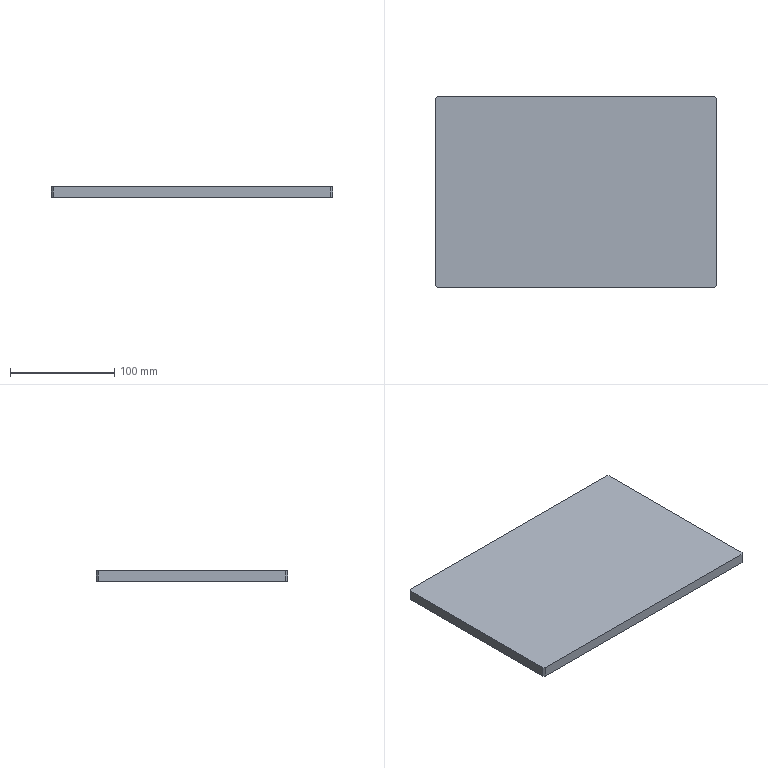Part | STEP file | 001-011-Blanking flip base plate | 1 solid | 10 faces | box 270 x 184 x 10 mm | volume 496720 mm3 | plane 10
STEP:
#1=CARTESIAN_POINT('',(0.,0.,0.));
#2=DIRECTION('',(0.,0.,1.));
#3=DIRECTION('',(1.,0.,0.));
#4=AXIS2_PLACEMENT_3D('',#1,#2,#3);
#5=CARTESIAN_POINT('',(135.,-90.,10.));
#6=VERTEX_POINT('',#5);
#7=CARTESIAN_POINT('',(135.,90.,10.));
#8=VERTEX_POINT('',#7);
#9=CARTESIAN_POINT('',(135.,-92.,10.));
#10=DIRECTION('',(0.,1.,0.));
#11=VECTOR('',#10,1.);
#12=LINE('',#9,#11);
#13=CARTESIAN_POINT('',(135.,-92.,10.));
#14=DIRECTION('',(-1.,0.,0.));
#15=DIRECTION('',(0.,-1.,0.));
#16=AXIS2_PLACEMENT_3D('',#13,#14,#15);
#17=PLANE('',#16);
#18=CARTESIAN_POINT('',(0.,0.));
#19=DIRECTION('',(-1.,0.));
#20=VECTOR('',#19,1.);
#21=LINE('',#18,#20);
#22=(GEOMETRIC_REPRESENTATION_CONTEXT(2)PARAMETRIC_REPRESENTATION_CONTEXT()REPRESENTATION_CONTEXT('',''));
#23=DEFINITIONAL_REPRESENTATION('',(#21),#22);
#24=PCURVE('',#17,#23);
#25=CARTESIAN_POINT('',(0.,0.,10.));
#26=DIRECTION('',(0.,0.,-1.));
#27=DIRECTION('',(-1.,0.,0.));
#28=AXIS2_PLACEMENT_3D('',#25,#26,#27);
#29=PLANE('',#28);
#30=CARTESIAN_POINT('',(-135.,-92.));
#31=DIRECTION('',(0.,1.));
#32=VECTOR('',#31,1.);
#33=LINE('',#30,#32);
#34=(GEOMETRIC_REPRESENTATION_CONTEXT(2)PARAMETRIC_REPRESENTATION_CONTEXT()REPRESENTATION_CONTEXT('',''));
#35=DEFINITIONAL_REPRESENTATION('',(#33),#34);
#36=PCURVE('',#29,#35);
#37=SURFACE_CURVE('',#12,(#24,#36),.PCURVE_S1.);
#38=EDGE_CURVE('',#6,#8,#37,.T.);
#39=ORIENTED_EDGE('',*,*,#38,.F.);
#40=CARTESIAN_POINT('',(135.,-90.,0.));
#41=VERTEX_POINT('',#40);
#42=CARTESIAN_POINT('',(135.,-90.,10.));
#43=DIRECTION('',(0.,0.,-1.));
#44=VECTOR('',#43,1.);
#45=LINE('',#42,#44);
#46=CARTESIAN_POINT('',(-2.,0.));
#47=DIRECTION('',(0.,-1.));
#48=VECTOR('',#47,1.);
#49=LINE('',#46,#48);
#50=(GEOMETRIC_REPRESENTATION_CONTEXT(2)PARAMETRIC_REPRESENTATION_CONTEXT()REPRESENTATION_CONTEXT('',''));
#51=DEFINITIONAL_REPRESENTATION('',(#49),#50);
#52=PCURVE('',#17,#51);
#53=CARTESIAN_POINT('',(135.,-90.,10.));
#54=DIRECTION('',(-0.7071,0.7071,0.));
#55=DIRECTION('',(0.,0.,-1.));
#56=AXIS2_PLACEMENT_3D('',#53,#54,#55);
#57=PLANE('',#56);
#58=CARTESIAN_POINT('',(0.,0.));
#59=DIRECTION('',(1.,0.));
#60=VECTOR('',#59,1.);
#61=LINE('',#58,#60);
#62=(GEOMETRIC_REPRESENTATION_CONTEXT(2)PARAMETRIC_REPRESENTATION_CONTEXT()REPRESENTATION_CONTEXT('',''));
#63=DEFINITIONAL_REPRESENTATION('',(#61),#62);
#64=PCURVE('',#57,#63);
#65=SURFACE_CURVE('',#45,(#52,#64),.PCURVE_S1.);
#66=EDGE_CURVE('',#6,#41,#65,.T.);
#67=ORIENTED_EDGE('',*,*,#66,.T.);
#68=CARTESIAN_POINT('',(135.,90.,0.));
#69=VERTEX_POINT('',#68);
#70=CARTESIAN_POINT('',(135.,-92.,0.));
#71=DIRECTION('',(0.,1.,0.));
#72=VECTOR('',#71,1.);
#73=LINE('',#70,#72);
#74=CARTESIAN_POINT('',(0.,-10.));
#75=DIRECTION('',(-1.,0.));
#76=VECTOR('',#75,1.);
#77=LINE('',#74,#76);
#78=(GEOMETRIC_REPRESENTATION_CONTEXT(2)PARAMETRIC_REPRESENTATION_CONTEXT()REPRESENTATION_CONTEXT('',''));
#79=DEFINITIONAL_REPRESENTATION('',(#77),#78);
#80=PCURVE('',#17,#79);
#81=CARTESIAN_POINT('',(0.,0.,0.));
#82=DIRECTION('',(0.,0.,-1.));
#83=DIRECTION('',(-1.,0.,0.));
#84=AXIS2_PLACEMENT_3D('',#81,#82,#83);
#85=PLANE('',#84);
#86=CARTESIAN_POINT('',(-135.,-92.));
#87=DIRECTION('',(0.,1.));
#88=VECTOR('',#87,1.);
#89=LINE('',#86,#88);
#90=(GEOMETRIC_REPRESENTATION_CONTEXT(2)PARAMETRIC_REPRESENTATION_CONTEXT()REPRESENTATION_CONTEXT('',''));
#91=DEFINITIONAL_REPRESENTATION('',(#89),#90);
#92=PCURVE('',#85,#91);
#93=SURFACE_CURVE('',#73,(#80,#92),.PCURVE_S1.);
#94=EDGE_CURVE('',#41,#69,#93,.T.);
#95=ORIENTED_EDGE('',*,*,#94,.T.);
#96=CARTESIAN_POINT('',(135.,90.,10.));
#97=DIRECTION('',(0.,0.,1.));
#98=VECTOR('',#97,1.);
#99=LINE('',#96,#98);
#100=CARTESIAN_POINT('',(-182.,0.));
#101=DIRECTION('',(0.,1.));
#102=VECTOR('',#101,1.);
#103=LINE('',#100,#102);
#104=(GEOMETRIC_REPRESENTATION_CONTEXT(2)PARAMETRIC_REPRESENTATION_CONTEXT()REPRESENTATION_CONTEXT('',''));
#105=DEFINITIONAL_REPRESENTATION('',(#103),#104);
#106=PCURVE('',#17,#105);
#107=CARTESIAN_POINT('',(133.,92.,10.));
#108=DIRECTION('',(-0.7071,-0.7071,0.));
#109=DIRECTION('',(0.,0.,-1.));
#110=AXIS2_PLACEMENT_3D('',#107,#108,#109);
#111=PLANE('',#110);
#112=CARTESIAN_POINT('',(0.,2.828));
#113=DIRECTION('',(-1.,0.));
#114=VECTOR('',#113,1.);
#115=LINE('',#112,#114);
#116=(GEOMETRIC_REPRESENTATION_CONTEXT(2)PARAMETRIC_REPRESENTATION_CONTEXT()REPRESENTATION_CONTEXT('',''));
#117=DEFINITIONAL_REPRESENTATION('',(#115),#116);
#118=PCURVE('',#111,#117);
#119=SURFACE_CURVE('',#99,(#106,#118),.PCURVE_S1.);
#120=EDGE_CURVE('',#69,#8,#119,.T.);
#121=ORIENTED_EDGE('',*,*,#120,.T.);
#122=EDGE_LOOP('',(#39,#67,#95,#121));
#123=FACE_BOUND('',#122,.T.);
#124=ADVANCED_FACE('',(#123),#17,.F.);
#125=CARTESIAN_POINT('',(133.,92.,10.));
#126=VERTEX_POINT('',#125);
#127=CARTESIAN_POINT('',(-133.,92.,10.));
#128=VERTEX_POINT('',#127);
#129=CARTESIAN_POINT('',(-135.,92.,10.));
#130=DIRECTION('',(-1.,0.,0.));
#131=VECTOR('',#130,1.);
#132=LINE('',#129,#131);
#133=CARTESIAN_POINT('',(-135.,92.,10.));
#134=DIRECTION('',(0.,-1.,0.));
#135=DIRECTION('',(0.,0.,-1.));
#136=AXIS2_PLACEMENT_3D('',#133,#134,#135);
#137=PLANE('',#136);
#138=CARTESIAN_POINT('',(0.,0.));
#139=DIRECTION('',(0.,-1.));
#140=VECTOR('',#139,1.);
#141=LINE('',#138,#140);
#142=(GEOMETRIC_REPRESENTATION_CONTEXT(2)PARAMETRIC_REPRESENTATION_CONTEXT()REPRESENTATION_CONTEXT('',''));
#143=DEFINITIONAL_REPRESENTATION('',(#141),#142);
#144=PCURVE('',#137,#143);
#145=CARTESIAN_POINT('',(135.,92.));
#146=DIRECTION('',(1.,0.));
#147=VECTOR('',#146,1.);
#148=LINE('',#145,#147);
#149=(GEOMETRIC_REPRESENTATION_CONTEXT(2)PARAMETRIC_REPRESENTATION_CONTEXT()REPRESENTATION_CONTEXT('',''));
#150=DEFINITIONAL_REPRESENTATION('',(#148),#149);
#151=PCURVE('',#29,#150);
#152=SURFACE_CURVE('',#132,(#144,#151),.PCURVE_S1.);
#153=EDGE_CURVE('',#126,#128,#152,.T.);
#154=ORIENTED_EDGE('',*,*,#153,.F.);
#155=CARTESIAN_POINT('',(133.,92.,0.));
#156=VERTEX_POINT('',#155);
#157=CARTESIAN_POINT('',(133.,92.,10.));
#158=DIRECTION('',(0.,0.,-1.));
#159=VECTOR('',#158,1.);
#160=LINE('',#157,#159);
#161=CARTESIAN_POINT('',(0.,268.));
#162=DIRECTION('',(1.,0.));
#163=VECTOR('',#162,1.);
#164=LINE('',#161,#163);
#165=(GEOMETRIC_REPRESENTATION_CONTEXT(2)PARAMETRIC_REPRESENTATION_CONTEXT()REPRESENTATION_CONTEXT('',''));
#166=DEFINITIONAL_REPRESENTATION('',(#164),#165);
#167=PCURVE('',#137,#166);
#168=CARTESIAN_POINT('',(0.,0.));
#169=DIRECTION('',(1.,0.));
#170=VECTOR('',#169,1.);
#171=LINE('',#168,#170);
#172=(GEOMETRIC_REPRESENTATION_CONTEXT(2)PARAMETRIC_REPRESENTATION_CONTEXT()REPRESENTATION_CONTEXT('',''));
#173=DEFINITIONAL_REPRESENTATION('',(#171),#172);
#174=PCURVE('',#111,#173);
#175=SURFACE_CURVE('',#160,(#167,#174),.PCURVE_S1.);
#176=EDGE_CURVE('',#126,#156,#175,.T.);
#177=ORIENTED_EDGE('',*,*,#176,.T.);
#178=CARTESIAN_POINT('',(-133.,92.,0.));
#179=VERTEX_POINT('',#178);
#180=CARTESIAN_POINT('',(-135.,92.,0.));
#181=DIRECTION('',(-1.,0.,0.));
#182=VECTOR('',#181,1.);
#183=LINE('',#180,#182);
#184=CARTESIAN_POINT('',(10.,0.));
#185=DIRECTION('',(0.,-1.));
#186=VECTOR('',#185,1.);
#187=LINE('',#184,#186);
#188=(GEOMETRIC_REPRESENTATION_CONTEXT(2)PARAMETRIC_REPRESENTATION_CONTEXT()REPRESENTATION_CONTEXT('',''));
#189=DEFINITIONAL_REPRESENTATION('',(#187),#188);
#190=PCURVE('',#137,#189);
#191=CARTESIAN_POINT('',(135.,92.));
#192=DIRECTION('',(1.,0.));
#193=VECTOR('',#192,1.);
#194=LINE('',#191,#193);
#195=(GEOMETRIC_REPRESENTATION_CONTEXT(2)PARAMETRIC_REPRESENTATION_CONTEXT()REPRESENTATION_CONTEXT('',''));
#196=DEFINITIONAL_REPRESENTATION('',(#194),#195);
#197=PCURVE('',#85,#196);
#198=SURFACE_CURVE('',#183,(#190,#197),.PCURVE_S1.);
#199=EDGE_CURVE('',#156,#179,#198,.T.);
#200=ORIENTED_EDGE('',*,*,#199,.T.);
#201=CARTESIAN_POINT('',(-133.,92.,10.));
#202=DIRECTION('',(0.,0.,1.));
#203=VECTOR('',#202,1.);
#204=LINE('',#201,#203);
#205=CARTESIAN_POINT('',(0.,2.));
#206=DIRECTION('',(-1.,0.));
#207=VECTOR('',#206,1.);
#208=LINE('',#205,#207);
#209=(GEOMETRIC_REPRESENTATION_CONTEXT(2)PARAMETRIC_REPRESENTATION_CONTEXT()REPRESENTATION_CONTEXT('',''));
#210=DEFINITIONAL_REPRESENTATION('',(#208),#209);
#211=PCURVE('',#137,#210);
#212=CARTESIAN_POINT('',(-135.,90.,10.));
#213=DIRECTION('',(0.7071,-0.7071,0.));
#214=DIRECTION('',(0.,0.,-1.));
#215=AXIS2_PLACEMENT_3D('',#212,#213,#214);
#216=PLANE('',#215);
#217=CARTESIAN_POINT('',(0.,2.828));
#218=DIRECTION('',(-1.,0.));
#219=VECTOR('',#218,1.);
#220=LINE('',#217,#219);
#221=(GEOMETRIC_REPRESENTATION_CONTEXT(2)PARAMETRIC_REPRESENTATION_CONTEXT()REPRESENTATION_CONTEXT('',''));
#222=DEFINITIONAL_REPRESENTATION('',(#220),#221);
#223=PCURVE('',#216,#222);
#224=SURFACE_CURVE('',#204,(#211,#223),.PCURVE_S1.);
#225=EDGE_CURVE('',#179,#128,#224,.T.);
#226=ORIENTED_EDGE('',*,*,#225,.T.);
#227=EDGE_LOOP('',(#154,#177,#200,#226));
#228=FACE_BOUND('',#227,.T.);
#229=ADVANCED_FACE('',(#228),#137,.F.);
#230=CARTESIAN_POINT('',(-135.,90.,0.));
#231=VERTEX_POINT('',#230);
#232=CARTESIAN_POINT('',(-135.,-90.,0.));
#233=VERTEX_POINT('',#232);
#234=CARTESIAN_POINT('',(-135.,-92.,0.));
#235=DIRECTION('',(0.,-1.,0.));
#236=VECTOR('',#235,1.);
#237=LINE('',#234,#236);
#238=CARTESIAN_POINT('',(-135.,-92.,10.));
#239=DIRECTION('',(1.,0.,0.));
#240=DIRECTION('',(0.,1.,0.));
#241=AXIS2_PLACEMENT_3D('',#238,#239,#240);
#242=PLANE('',#241);
#243=CARTESIAN_POINT('',(0.,-10.));
#244=DIRECTION('',(-1.,0.));
#245=VECTOR('',#244,1.);
#246=LINE('',#243,#245);
#247=(GEOMETRIC_REPRESENTATION_CONTEXT(2)PARAMETRIC_REPRESENTATION_CONTEXT()REPRESENTATION_CONTEXT('',''));
#248=DEFINITIONAL_REPRESENTATION('',(#246),#247);
#249=PCURVE('',#242,#248);
#250=CARTESIAN_POINT('',(135.,-92.));
#251=DIRECTION('',(0.,-1.));
#252=VECTOR('',#251,1.);
#253=LINE('',#250,#252);
#254=(GEOMETRIC_REPRESENTATION_CONTEXT(2)PARAMETRIC_REPRESENTATION_CONTEXT()REPRESENTATION_CONTEXT('',''));
#255=DEFINITIONAL_REPRESENTATION('',(#253),#254);
#256=PCURVE('',#85,#255);
#257=SURFACE_CURVE('',#237,(#249,#256),.PCURVE_S1.);
#258=EDGE_CURVE('',#231,#233,#257,.T.);
#259=ORIENTED_EDGE('',*,*,#258,.T.);
#260=CARTESIAN_POINT('',(-135.,-90.,10.));
#261=VERTEX_POINT('',#260);
#262=CARTESIAN_POINT('',(-135.,-90.,10.));
#263=DIRECTION('',(0.,0.,1.));
#264=VECTOR('',#263,1.);
#265=LINE('',#262,#264);
#266=CARTESIAN_POINT('',(2.,0.));
#267=DIRECTION('',(0.,1.));
#268=VECTOR('',#267,1.);
#269=LINE('',#266,#268);
#270=(GEOMETRIC_REPRESENTATION_CONTEXT(2)PARAMETRIC_REPRESENTATION_CONTEXT()REPRESENTATION_CONTEXT('',''));
#271=DEFINITIONAL_REPRESENTATION('',(#269),#270);
#272=PCURVE('',#242,#271);
#273=CARTESIAN_POINT('',(-133.,-92.,10.));
#274=DIRECTION('',(0.7071,0.7071,0.));
#275=DIRECTION('',(0.,0.,-1.));
#276=AXIS2_PLACEMENT_3D('',#273,#274,#275);
#277=PLANE('',#276);
#278=CARTESIAN_POINT('',(0.,2.828));
#279=DIRECTION('',(-1.,0.));
#280=VECTOR('',#279,1.);
#281=LINE('',#278,#280);
#282=(GEOMETRIC_REPRESENTATION_CONTEXT(2)PARAMETRIC_REPRESENTATION_CONTEXT()REPRESENTATION_CONTEXT('',''));
#283=DEFINITIONAL_REPRESENTATION('',(#281),#282);
#284=PCURVE('',#277,#283);
#285=SURFACE_CURVE('',#265,(#272,#284),.PCURVE_S1.);
#286=EDGE_CURVE('',#233,#261,#285,.T.);
#287=ORIENTED_EDGE('',*,*,#286,.T.);
#288=CARTESIAN_POINT('',(-135.,90.,10.));
#289=VERTEX_POINT('',#288);
#290=CARTESIAN_POINT('',(-135.,-92.,10.));
#291=DIRECTION('',(0.,-1.,0.));
#292=VECTOR('',#291,1.);
#293=LINE('',#290,#292);
#294=CARTESIAN_POINT('',(0.,0.));
#295=DIRECTION('',(-1.,0.));
#296=VECTOR('',#295,1.);
#297=LINE('',#294,#296);
#298=(GEOMETRIC_REPRESENTATION_CONTEXT(2)PARAMETRIC_REPRESENTATION_CONTEXT()REPRESENTATION_CONTEXT('',''));
#299=DEFINITIONAL_REPRESENTATION('',(#297),#298);
#300=PCURVE('',#242,#299);
#301=CARTESIAN_POINT('',(135.,-92.));
#302=DIRECTION('',(0.,-1.));
#303=VECTOR('',#302,1.);
#304=LINE('',#301,#303);
#305=(GEOMETRIC_REPRESENTATION_CONTEXT(2)PARAMETRIC_REPRESENTATION_CONTEXT()REPRESENTATION_CONTEXT('',''));
#306=DEFINITIONAL_REPRESENTATION('',(#304),#305);
#307=PCURVE('',#29,#306);
#308=SURFACE_CURVE('',#293,(#300,#307),.PCURVE_S1.);
#309=EDGE_CURVE('',#289,#261,#308,.T.);
#310=ORIENTED_EDGE('',*,*,#309,.F.);
#311=CARTESIAN_POINT('',(-135.,90.,10.));
#312=DIRECTION('',(0.,0.,-1.));
#313=VECTOR('',#312,1.);
#314=LINE('',#311,#313);
#315=CARTESIAN_POINT('',(182.,0.));
#316=DIRECTION('',(0.,-1.));
#317=VECTOR('',#316,1.);
#318=LINE('',#315,#317);
#319=(GEOMETRIC_REPRESENTATION_CONTEXT(2)PARAMETRIC_REPRESENTATION_CONTEXT()REPRESENTATION_CONTEXT('',''));
#320=DEFINITIONAL_REPRESENTATION('',(#318),#319);
#321=PCURVE('',#242,#320);
#322=CARTESIAN_POINT('',(0.,0.));
#323=DIRECTION('',(1.,0.));
#324=VECTOR('',#323,1.);
#325=LINE('',#322,#324);
#326=(GEOMETRIC_REPRESENTATION_CONTEXT(2)PARAMETRIC_REPRESENTATION_CONTEXT()REPRESENTATION_CONTEXT('',''));
#327=DEFINITIONAL_REPRESENTATION('',(#325),#326);
#328=PCURVE('',#216,#327);
#329=SURFACE_CURVE('',#314,(#321,#328),.PCURVE_S1.);
#330=EDGE_CURVE('',#289,#231,#329,.T.);
#331=ORIENTED_EDGE('',*,*,#330,.T.);
#332=EDGE_LOOP('',(#259,#287,#310,#331));
#333=FACE_BOUND('',#332,.T.);
#334=ADVANCED_FACE('',(#333),#242,.F.);
#335=CARTESIAN_POINT('',(-133.,-92.,0.));
#336=VERTEX_POINT('',#335);
#337=CARTESIAN_POINT('',(133.,-92.,0.));
#338=VERTEX_POINT('',#337);
#339=CARTESIAN_POINT('',(-135.,-92.,0.));
#340=DIRECTION('',(1.,0.,0.));
#341=VECTOR('',#340,1.);
#342=LINE('',#339,#341);
#343=CARTESIAN_POINT('',(-135.,-92.,10.));
#344=DIRECTION('',(0.,1.,0.));
#345=DIRECTION('',(0.,0.,1.));
#346=AXIS2_PLACEMENT_3D('',#343,#344,#345);
#347=PLANE('',#346);
#348=CARTESIAN_POINT('',(-10.,0.));
#349=DIRECTION('',(0.,1.));
#350=VECTOR('',#349,1.);
#351=LINE('',#348,#350);
#352=(GEOMETRIC_REPRESENTATION_CONTEXT(2)PARAMETRIC_REPRESENTATION_CONTEXT()REPRESENTATION_CONTEXT('',''));
#353=DEFINITIONAL_REPRESENTATION('',(#351),#352);
#354=PCURVE('',#347,#353);
#355=CARTESIAN_POINT('',(135.,-92.));
#356=DIRECTION('',(-1.,0.));
#357=VECTOR('',#356,1.);
#358=LINE('',#355,#357);
#359=(GEOMETRIC_REPRESENTATION_CONTEXT(2)PARAMETRIC_REPRESENTATION_CONTEXT()REPRESENTATION_CONTEXT('',''));
#360=DEFINITIONAL_REPRESENTATION('',(#358),#359);
#361=PCURVE('',#85,#360);
#362=SURFACE_CURVE('',#342,(#354,#361),.PCURVE_S1.);
#363=EDGE_CURVE('',#336,#338,#362,.T.);
#364=ORIENTED_EDGE('',*,*,#363,.T.);
#365=CARTESIAN_POINT('',(133.,-92.,10.));
#366=VERTEX_POINT('',#365);
#367=CARTESIAN_POINT('',(133.,-92.,10.));
#368=DIRECTION('',(0.,0.,1.));
#369=VECTOR('',#368,1.);
#370=LINE('',#367,#369);
#371=CARTESIAN_POINT('',(0.,268.));
#372=DIRECTION('',(1.,0.));
#373=VECTOR('',#372,1.);
#374=LINE('',#371,#373);
#375=(GEOMETRIC_REPRESENTATION_CONTEXT(2)PARAMETRIC_REPRESENTATION_CONTEXT()REPRESENTATION_CONTEXT('',''));
#376=DEFINITIONAL_REPRESENTATION('',(#374),#375);
#377=PCURVE('',#347,#376);
#378=CARTESIAN_POINT('',(0.,2.828));
#379=DIRECTION('',(-1.,0.));
#380=VECTOR('',#379,1.);
#381=LINE('',#378,#380);
#382=(GEOMETRIC_REPRESENTATION_CONTEXT(2)PARAMETRIC_REPRESENTATION_CONTEXT()REPRESENTATION_CONTEXT('',''));
#383=DEFINITIONAL_REPRESENTATION('',(#381),#382);
#384=PCURVE('',#57,#383);
#385=SURFACE_CURVE('',#370,(#377,#384),.PCURVE_S1.);
#386=EDGE_CURVE('',#338,#366,#385,.T.);
#387=ORIENTED_EDGE('',*,*,#386,.T.);
#388=CARTESIAN_POINT('',(-133.,-92.,10.));
#389=VERTEX_POINT('',#388);
#390=CARTESIAN_POINT('',(-135.,-92.,10.));
#391=DIRECTION('',(1.,0.,0.));
#392=VECTOR('',#391,1.);
#393=LINE('',#390,#392);
#394=CARTESIAN_POINT('',(0.,0.));
#395=DIRECTION('',(0.,1.));
#396=VECTOR('',#395,1.);
#397=LINE('',#394,#396);
#398=(GEOMETRIC_REPRESENTATION_CONTEXT(2)PARAMETRIC_REPRESENTATION_CONTEXT()REPRESENTATION_CONTEXT('',''));
#399=DEFINITIONAL_REPRESENTATION('',(#397),#398);
#400=PCURVE('',#347,#399);
#401=CARTESIAN_POINT('',(135.,-92.));
#402=DIRECTION('',(-1.,0.));
#403=VECTOR('',#402,1.);
#404=LINE('',#401,#403);
#405=(GEOMETRIC_REPRESENTATION_CONTEXT(2)PARAMETRIC_REPRESENTATION_CONTEXT()REPRESENTATION_CONTEXT('',''));
#406=DEFINITIONAL_REPRESENTATION('',(#404),#405);
#407=PCURVE('',#29,#406);
#408=SURFACE_CURVE('',#393,(#400,#407),.PCURVE_S1.);
#409=EDGE_CURVE('',#389,#366,#408,.T.);
#410=ORIENTED_EDGE('',*,*,#409,.F.);
#411=CARTESIAN_POINT('',(-133.,-92.,10.));
#412=DIRECTION('',(0.,0.,-1.));
#413=VECTOR('',#412,1.);
#414=LINE('',#411,#413);
#415=CARTESIAN_POINT('',(0.,2.));
#416=DIRECTION('',(-1.,0.));
#417=VECTOR('',#416,1.);
#418=LINE('',#415,#417);
#419=(GEOMETRIC_REPRESENTATION_CONTEXT(2)PARAMETRIC_REPRESENTATION_CONTEXT()REPRESENTATION_CONTEXT('',''));
#420=DEFINITIONAL_REPRESENTATION('',(#418),#419);
#421=PCURVE('',#347,#420);
#422=CARTESIAN_POINT('',(0.,0.));
#423=DIRECTION('',(1.,0.));
#424=VECTOR('',#423,1.);
#425=LINE('',#422,#424);
#426=(GEOMETRIC_REPRESENTATION_CONTEXT(2)PARAMETRIC_REPRESENTATION_CONTEXT()REPRESENTATION_CONTEXT('',''));
#427=DEFINITIONAL_REPRESENTATION('',(#425),#426);
#428=PCURVE('',#277,#427);
#429=SURFACE_CURVE('',#414,(#421,#428),.PCURVE_S1.);
#430=EDGE_CURVE('',#389,#336,#429,.T.);
#431=ORIENTED_EDGE('',*,*,#430,.T.);
#432=EDGE_LOOP('',(#364,#387,#410,#431));
#433=FACE_BOUND('',#432,.T.);
#434=ADVANCED_FACE('',(#433),#347,.F.);
#435=ORIENTED_EDGE('',*,*,#409,.T.);
#436=CARTESIAN_POINT('',(135.,-90.,10.));
#437=DIRECTION('',(0.7071,0.7071,0.));
#438=VECTOR('',#437,1.);
#439=LINE('',#436,#438);
#440=CARTESIAN_POINT('',(-135.,-90.));
#441=DIRECTION('',(-0.7071,0.7071));
#442=VECTOR('',#441,1.);
#443=LINE('',#440,#442);
#444=(GEOMETRIC_REPRESENTATION_CONTEXT(2)PARAMETRIC_REPRESENTATION_CONTEXT()REPRESENTATION_CONTEXT('',''));
#445=DEFINITIONAL_REPRESENTATION('',(#443),#444);
#446=PCURVE('',#29,#445);
#447=CARTESIAN_POINT('',(0.,0.));
#448=DIRECTION('',(0.,-1.));
#449=VECTOR('',#448,1.);
#450=LINE('',#447,#449);
#451=(GEOMETRIC_REPRESENTATION_CONTEXT(2)PARAMETRIC_REPRESENTATION_CONTEXT()REPRESENTATION_CONTEXT('',''));
#452=DEFINITIONAL_REPRESENTATION('',(#450),#451);
#453=PCURVE('',#57,#452);
#454=SURFACE_CURVE('',#439,(#446,#453),.PCURVE_S1.);
#455=EDGE_CURVE('',#366,#6,#454,.T.);
#456=ORIENTED_EDGE('',*,*,#455,.T.);
#457=ORIENTED_EDGE('',*,*,#38,.T.);
#458=CARTESIAN_POINT('',(133.,92.,10.));
#459=DIRECTION('',(-0.7071,0.7071,0.));
#460=VECTOR('',#459,1.);
#461=LINE('',#458,#460);
#462=CARTESIAN_POINT('',(-133.,92.));
#463=DIRECTION('',(0.7071,0.7071));
#464=VECTOR('',#463,1.);
#465=LINE('',#462,#464);
#466=(GEOMETRIC_REPRESENTATION_CONTEXT(2)PARAMETRIC_REPRESENTATION_CONTEXT()REPRESENTATION_CONTEXT('',''));
#467=DEFINITIONAL_REPRESENTATION('',(#465),#466);
#468=PCURVE('',#29,#467);
#469=CARTESIAN_POINT('',(0.,0.));
#470=DIRECTION('',(0.,-1.));
#471=VECTOR('',#470,1.);
#472=LINE('',#469,#471);
#473=(GEOMETRIC_REPRESENTATION_CONTEXT(2)PARAMETRIC_REPRESENTATION_CONTEXT()REPRESENTATION_CONTEXT('',''));
#474=DEFINITIONAL_REPRESENTATION('',(#472),#473);
#475=PCURVE('',#111,#474);
#476=SURFACE_CURVE('',#461,(#468,#475),.PCURVE_S1.);
#477=EDGE_CURVE('',#8,#126,#476,.T.);
#478=ORIENTED_EDGE('',*,*,#477,.T.);
#479=ORIENTED_EDGE('',*,*,#153,.T.);
#480=CARTESIAN_POINT('',(-135.,90.,10.));
#481=DIRECTION('',(-0.7071,-0.7071,0.));
#482=VECTOR('',#481,1.);
#483=LINE('',#480,#482);
#484=CARTESIAN_POINT('',(135.,90.));
#485=DIRECTION('',(0.7071,-0.7071));
#486=VECTOR('',#485,1.);
#487=LINE('',#484,#486);
#488=(GEOMETRIC_REPRESENTATION_CONTEXT(2)PARAMETRIC_REPRESENTATION_CONTEXT()REPRESENTATION_CONTEXT('',''));
#489=DEFINITIONAL_REPRESENTATION('',(#487),#488);
#490=PCURVE('',#29,#489);
#491=CARTESIAN_POINT('',(0.,0.));
#492=DIRECTION('',(0.,-1.));
#493=VECTOR('',#492,1.);
#494=LINE('',#491,#493);
#495=(GEOMETRIC_REPRESENTATION_CONTEXT(2)PARAMETRIC_REPRESENTATION_CONTEXT()REPRESENTATION_CONTEXT('',''));
#496=DEFINITIONAL_REPRESENTATION('',(#494),#495);
#497=PCURVE('',#216,#496);
#498=SURFACE_CURVE('',#483,(#490,#497),.PCURVE_S1.);
#499=EDGE_CURVE('',#128,#289,#498,.T.);
#500=ORIENTED_EDGE('',*,*,#499,.T.);
#501=ORIENTED_EDGE('',*,*,#309,.T.);
#502=CARTESIAN_POINT('',(-133.,-92.,10.));
#503=DIRECTION('',(0.7071,-0.7071,0.));
#504=VECTOR('',#503,1.);
#505=LINE('',#502,#504);
#506=CARTESIAN_POINT('',(133.,-92.));
#507=DIRECTION('',(-0.7071,-0.7071));
#508=VECTOR('',#507,1.);
#509=LINE('',#506,#508);
#510=(GEOMETRIC_REPRESENTATION_CONTEXT(2)PARAMETRIC_REPRESENTATION_CONTEXT()REPRESENTATION_CONTEXT('',''));
#511=DEFINITIONAL_REPRESENTATION('',(#509),#510);
#512=PCURVE('',#29,#511);
#513=CARTESIAN_POINT('',(0.,0.));
#514=DIRECTION('',(0.,-1.));
#515=VECTOR('',#514,1.);
#516=LINE('',#513,#515);
#517=(GEOMETRIC_REPRESENTATION_CONTEXT(2)PARAMETRIC_REPRESENTATION_CONTEXT()REPRESENTATION_CONTEXT('',''));
#518=DEFINITIONAL_REPRESENTATION('',(#516),#517);
#519=PCURVE('',#277,#518);
#520=SURFACE_CURVE('',#505,(#512,#519),.PCURVE_S1.);
#521=EDGE_CURVE('',#261,#389,#520,.T.);
#522=ORIENTED_EDGE('',*,*,#521,.T.);
#523=EDGE_LOOP('',(#435,#456,#457,#478,#479,#500,#501,#522));
#524=FACE_BOUND('',#523,.T.);
#525=ADVANCED_FACE('',(#524),#29,.F.);
#526=ORIENTED_EDGE('',*,*,#94,.F.);
#527=CARTESIAN_POINT('',(112.5,-112.5,0.));
#528=DIRECTION('',(-0.7071,-0.7071,0.));
#529=VECTOR('',#528,1.);
#530=LINE('',#527,#529);
#531=CARTESIAN_POINT('',(-112.5,-112.5));
#532=DIRECTION('',(0.7071,-0.7071));
#533=VECTOR('',#532,1.);
#534=LINE('',#531,#533);
#535=(GEOMETRIC_REPRESENTATION_CONTEXT(2)PARAMETRIC_REPRESENTATION_CONTEXT()REPRESENTATION_CONTEXT('',''));
#536=DEFINITIONAL_REPRESENTATION('',(#534),#535);
#537=PCURVE('',#85,#536);
#538=CARTESIAN_POINT('',(10.,31.82));
#539=DIRECTION('',(0.,1.));
#540=VECTOR('',#539,1.);
#541=LINE('',#538,#540);
#542=(GEOMETRIC_REPRESENTATION_CONTEXT(2)PARAMETRIC_REPRESENTATION_CONTEXT()REPRESENTATION_CONTEXT('',''));
#543=DEFINITIONAL_REPRESENTATION('',(#541),#542);
#544=PCURVE('',#57,#543);
#545=SURFACE_CURVE('',#530,(#537,#544),.PCURVE_S1.);
#546=EDGE_CURVE('',#41,#338,#545,.T.);
#547=ORIENTED_EDGE('',*,*,#546,.T.);
#548=ORIENTED_EDGE('',*,*,#363,.F.);
#549=CARTESIAN_POINT('',(-112.5,-112.5,0.));
#550=DIRECTION('',(-0.7071,0.7071,0.));
#551=VECTOR('',#550,1.);
#552=LINE('',#549,#551);
#553=CARTESIAN_POINT('',(112.5,-112.5));
#554=DIRECTION('',(0.7071,0.7071));
#555=VECTOR('',#554,1.);
#556=LINE('',#553,#555);
#557=(GEOMETRIC_REPRESENTATION_CONTEXT(2)PARAMETRIC_REPRESENTATION_CONTEXT()REPRESENTATION_CONTEXT('',''));
#558=DEFINITIONAL_REPRESENTATION('',(#556),#557);
#559=PCURVE('',#85,#558);
#560=CARTESIAN_POINT('',(10.,-28.991));
#561=DIRECTION('',(0.,1.));
#562=VECTOR('',#561,1.);
#563=LINE('',#560,#562);
#564=(GEOMETRIC_REPRESENTATION_CONTEXT(2)PARAMETRIC_REPRESENTATION_CONTEXT()REPRESENTATION_CONTEXT('',''));
#565=DEFINITIONAL_REPRESENTATION('',(#563),#564);
#566=PCURVE('',#277,#565);
#567=SURFACE_CURVE('',#552,(#559,#566),.PCURVE_S1.);
#568=EDGE_CURVE('',#336,#233,#567,.T.);
#569=ORIENTED_EDGE('',*,*,#568,.T.);
#570=ORIENTED_EDGE('',*,*,#258,.F.);
#571=CARTESIAN_POINT('',(-112.5,112.5,0.));
#572=DIRECTION('',(0.7071,0.7071,0.));
#573=VECTOR('',#572,1.);
#574=LINE('',#571,#573);
#575=CARTESIAN_POINT('',(112.5,112.5));
#576=DIRECTION('',(-0.7071,0.7071));
#577=VECTOR('',#576,1.);
#578=LINE('',#575,#577);
#579=(GEOMETRIC_REPRESENTATION_CONTEXT(2)PARAMETRIC_REPRESENTATION_CONTEXT()REPRESENTATION_CONTEXT('',''));
#580=DEFINITIONAL_REPRESENTATION('',(#578),#579);
#581=PCURVE('',#85,#580);
#582=CARTESIAN_POINT('',(10.,31.82));
#583=DIRECTION('',(0.,1.));
#584=VECTOR('',#583,1.);
#585=LINE('',#582,#584);
#586=(GEOMETRIC_REPRESENTATION_CONTEXT(2)PARAMETRIC_REPRESENTATION_CONTEXT()REPRESENTATION_CONTEXT('',''));
#587=DEFINITIONAL_REPRESENTATION('',(#585),#586);
#588=PCURVE('',#216,#587);
#589=SURFACE_CURVE('',#574,(#581,#588),.PCURVE_S1.);
#590=EDGE_CURVE('',#231,#179,#589,.T.);
#591=ORIENTED_EDGE('',*,*,#590,.T.);
#592=ORIENTED_EDGE('',*,*,#199,.F.);
#593=CARTESIAN_POINT('',(112.5,112.5,0.));
#594=DIRECTION('',(0.7071,-0.7071,0.));
#595=VECTOR('',#594,1.);
#596=LINE('',#593,#595);
#597=CARTESIAN_POINT('',(-112.5,112.5));
#598=DIRECTION('',(-0.7071,-0.7071));
#599=VECTOR('',#598,1.);
#600=LINE('',#597,#599);
#601=(GEOMETRIC_REPRESENTATION_CONTEXT(2)PARAMETRIC_REPRESENTATION_CONTEXT()REPRESENTATION_CONTEXT('',''));
#602=DEFINITIONAL_REPRESENTATION('',(#600),#601);
#603=PCURVE('',#85,#602);
#604=CARTESIAN_POINT('',(10.,-28.991));
#605=DIRECTION('',(0.,1.));
#606=VECTOR('',#605,1.);
#607=LINE('',#604,#606);
#608=(GEOMETRIC_REPRESENTATION_CONTEXT(2)PARAMETRIC_REPRESENTATION_CONTEXT()REPRESENTATION_CONTEXT('',''));
#609=DEFINITIONAL_REPRESENTATION('',(#607),#608);
#610=PCURVE('',#111,#609);
#611=SURFACE_CURVE('',#596,(#603,#610),.PCURVE_S1.);
#612=EDGE_CURVE('',#156,#69,#611,.T.);
#613=ORIENTED_EDGE('',*,*,#612,.T.);
#614=EDGE_LOOP('',(#526,#547,#548,#569,#570,#591,#592,#613));
#615=FACE_BOUND('',#614,.T.);
#616=ADVANCED_FACE('',(#615),#85,.T.);
#617=ORIENTED_EDGE('',*,*,#455,.F.);
#618=ORIENTED_EDGE('',*,*,#386,.F.);
#619=ORIENTED_EDGE('',*,*,#546,.F.);
#620=ORIENTED_EDGE('',*,*,#66,.F.);
#621=EDGE_LOOP('',(#617,#618,#619,#620));
#622=FACE_BOUND('',#621,.T.);
#623=ADVANCED_FACE('',(#622),#57,.F.);
#624=ORIENTED_EDGE('',*,*,#521,.F.);
#625=ORIENTED_EDGE('',*,*,#286,.F.);
#626=ORIENTED_EDGE('',*,*,#568,.F.);
#627=ORIENTED_EDGE('',*,*,#430,.F.);
#628=EDGE_LOOP('',(#624,#625,#626,#627));
#629=FACE_BOUND('',#628,.T.);
#630=ADVANCED_FACE('',(#629),#277,.F.);
#631=ORIENTED_EDGE('',*,*,#477,.F.);
#632=ORIENTED_EDGE('',*,*,#120,.F.);
#633=ORIENTED_EDGE('',*,*,#612,.F.);
#634=ORIENTED_EDGE('',*,*,#176,.F.);
#635=EDGE_LOOP('',(#631,#632,#633,#634));
#636=FACE_BOUND('',#635,.T.);
#637=ADVANCED_FACE('',(#636),#111,.F.);
#638=ORIENTED_EDGE('',*,*,#499,.F.);
#639=ORIENTED_EDGE('',*,*,#225,.F.);
#640=ORIENTED_EDGE('',*,*,#590,.F.);
#641=ORIENTED_EDGE('',*,*,#330,.F.);
#642=EDGE_LOOP('',(#638,#639,#640,#641));
#643=FACE_BOUND('',#642,.T.);
#644=ADVANCED_FACE('',(#643),#216,.F.);
#645=CLOSED_SHELL('',(#124,#229,#334,#434,#525,#616,#623,#630,#637,#644));
#646=MANIFOLD_SOLID_BREP('',#645);
#647=(LENGTH_UNIT()NAMED_UNIT(*)SI_UNIT(.MILLI.,.METRE.));
#648=UNCERTAINTY_MEASURE_WITH_UNIT(LENGTH_MEASURE(0.0000001),#647,'','');
#649=(NAMED_UNIT(*)PLANE_ANGLE_UNIT()SI_UNIT($,.RADIAN.));
#650=(NAMED_UNIT(*)SI_UNIT($,.STERADIAN.)SOLID_ANGLE_UNIT());
#651=(GEOMETRIC_REPRESENTATION_CONTEXT(3)GLOBAL_UNCERTAINTY_ASSIGNED_CONTEXT((#648))GLOBAL_UNIT_ASSIGNED_CONTEXT((#647,#649,#650))REPRESENTATION_CONTEXT('',''));
#652=ADVANCED_BREP_SHAPE_REPRESENTATION('',(#4,#646),#651);